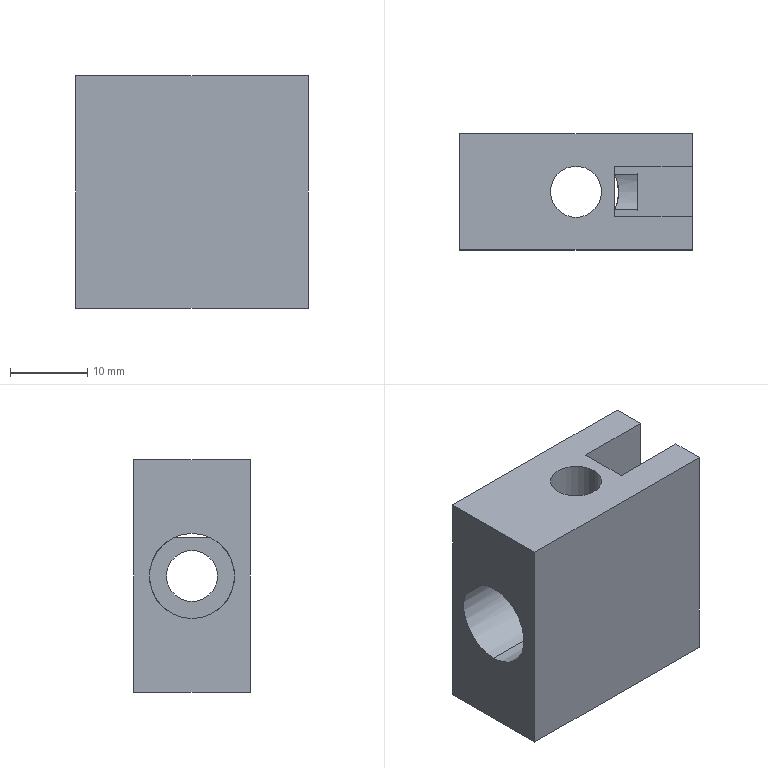Part | STEP file | Right-angle connecting block | 1 solid | 23 faces | box 30 x 15 x 30 mm | volume 8895 mm3 | plane 12 | cylinder 11 | commonest cylinder face diameters 11 x7 6.6 x4